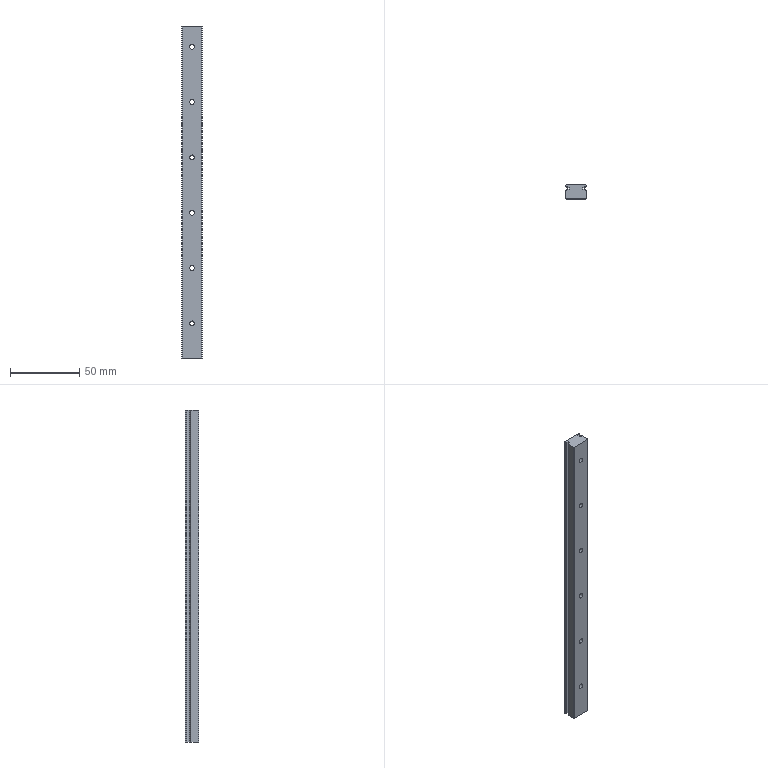Part | SolidWorks | 1 solid | 56 faces | box 15 x 10 x 240 mm | volume 32544 mm3 | cylinder 28 | plane 28 | commonest cylinder face diameters 3.5 x16 6 x12